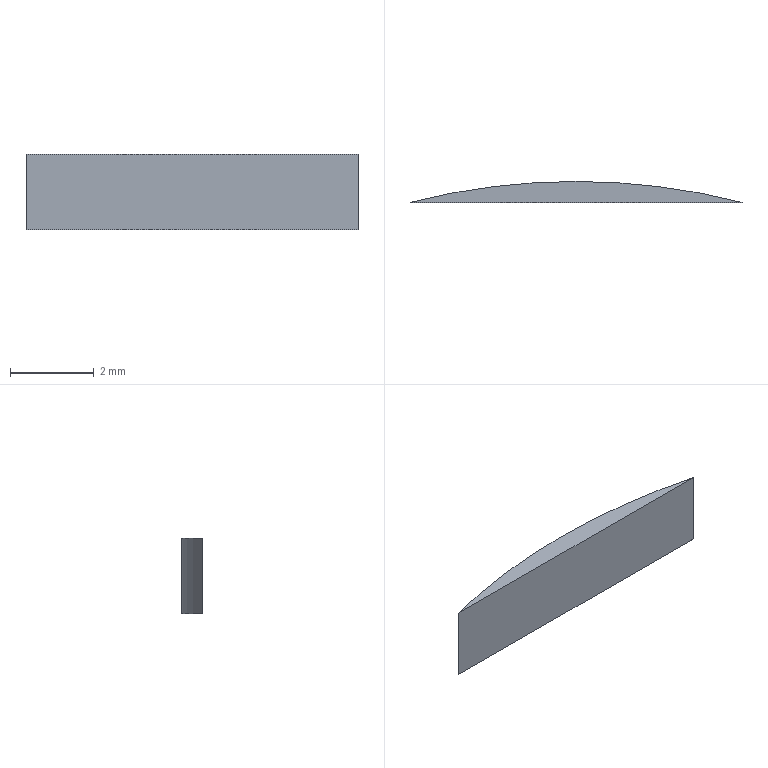Part | STEP file | ASND-0110-Q1-1 | 1 solid | 4 faces | box 7.937 x 0.5 x 1.8 mm | volume 4.777 mm3 | plane 3 | cylinder 1 | commonest cylinder face diameters 32 x1
STEP:
#1=CARTESIAN_POINT('',(0.,0.,0.));
#2=DIRECTION('',(0.,0.,1.));
#3=DIRECTION('',(1.,0.,0.));
#4=AXIS2_PLACEMENT_3D('',#1,#2,#3);
#5=CARTESIAN_POINT('',(2996.031,15.5,-129.5));
#6=VERTEX_POINT('',#5);
#7=CARTESIAN_POINT('',(2996.031,15.5,-127.7));
#8=VERTEX_POINT('',#7);
#9=CARTESIAN_POINT('',(2996.031,15.5,-128.6));
#10=DIRECTION('',(0.,0.,1.));
#11=VECTOR('',#10,1.);
#12=LINE('',#9,#11);
#13=CARTESIAN_POINT('',(3000.,0.,-128.6));
#14=DIRECTION('',(0.,0.,-1.));
#15=DIRECTION('',(-1.,0.,0.));
#16=AXIS2_PLACEMENT_3D('',#13,#14,#15);
#17=CYLINDRICAL_SURFACE('',#16,16.);
#18=CARTESIAN_POINT('',(1.32,0.));
#19=DIRECTION('',(0.,-1.));
#20=VECTOR('',#19,1.);
#21=LINE('',#18,#20);
#22=(GEOMETRIC_REPRESENTATION_CONTEXT(2)PARAMETRIC_REPRESENTATION_CONTEXT()REPRESENTATION_CONTEXT('',''));
#23=DEFINITIONAL_REPRESENTATION('',(#21),#22);
#24=PCURVE('',#17,#23);
#25=CARTESIAN_POINT('',(1241.605,15.5,-583.518));
#26=DIRECTION('',(0.,1.,0.));
#27=DIRECTION('',(0.7071,0.,0.7071));
#28=AXIS2_PLACEMENT_3D('',#25,#26,#27);
#29=PLANE('',#28);
#30=CARTESIAN_POINT('',(1562.242,918.891));
#31=DIRECTION('',(0.7071,-0.7071));
#32=VECTOR('',#31,1.);
#33=LINE('',#30,#32);
#34=(GEOMETRIC_REPRESENTATION_CONTEXT(2)PARAMETRIC_REPRESENTATION_CONTEXT()REPRESENTATION_CONTEXT('',''));
#35=DEFINITIONAL_REPRESENTATION('',(#33),#34);
#36=PCURVE('',#29,#35);
#37=SURFACE_CURVE('',#12,(#24,#36),.PCURVE_S1.);
#38=EDGE_CURVE('',#6,#8,#37,.T.);
#39=ORIENTED_EDGE('',*,*,#38,.T.);
#40=CARTESIAN_POINT('',(3003.969,15.5,-127.7));
#41=VERTEX_POINT('',#40);
#42=CARTESIAN_POINT('',(3000.,0.,-127.7));
#43=DIRECTION('',(0.,0.,-1.));
#44=DIRECTION('',(-1.,0.,0.));
#45=AXIS2_PLACEMENT_3D('',#42,#43,#44);
#46=CIRCLE('',#45,16.);
#47=CARTESIAN_POINT('',(0.,-0.9));
#48=DIRECTION('',(1.,0.));
#49=VECTOR('',#48,1.);
#50=LINE('',#47,#49);
#51=(GEOMETRIC_REPRESENTATION_CONTEXT(2)PARAMETRIC_REPRESENTATION_CONTEXT()REPRESENTATION_CONTEXT('',''));
#52=DEFINITIONAL_REPRESENTATION('',(#50),#51);
#53=PCURVE('',#17,#52);
#54=CARTESIAN_POINT('',(3000.,14.,-127.7));
#55=DIRECTION('',(0.,0.,1.));
#56=DIRECTION('',(0.7071,0.7071,0.));
#57=AXIS2_PLACEMENT_3D('',#54,#55,#56);
#58=PLANE('',#57);
#59=CARTESIAN_POINT('',(-21.213,1.414));
#60=CARTESIAN_POINT('',(-1.617,21.01));
#61=CARTESIAN_POINT('',(5.555,-5.758));
#62=CARTESIAN_POINT('',(12.728,-32.527));
#63=CARTESIAN_POINT('',(-14.041,-25.354));
#64=CARTESIAN_POINT('',(-40.809,-18.182));
#65=CARTESIAN_POINT('',(-21.213,1.414));
#66=(BOUNDED_CURVE()B_SPLINE_CURVE(2,(#59,#60,#61,#62,#63,#64,#65),.UNSPECIFIED.,.T.,.F.)B_SPLINE_CURVE_WITH_KNOTS((1,2,2,2,2,1),(-2.094,0.,2.094,4.189,6.283,8.378),.UNSPECIFIED.)CURVE()GEOMETRIC_REPRESENTATION_ITEM()RATIONAL_B_SPLINE_CURVE((1.,0.5,1.,0.5,1.,0.5,1.))REPRESENTATION_ITEM(''));
#67=(GEOMETRIC_REPRESENTATION_CONTEXT(2)PARAMETRIC_REPRESENTATION_CONTEXT()REPRESENTATION_CONTEXT('',''));
#68=DEFINITIONAL_REPRESENTATION('',(#66),#67);
#69=PCURVE('',#58,#68);
#70=SURFACE_CURVE('',#46,(#53,#69),.PCURVE_S1.);
#71=EDGE_CURVE('',#8,#41,#70,.T.);
#72=ORIENTED_EDGE('',*,*,#71,.T.);
#73=CARTESIAN_POINT('',(3003.969,15.5,-129.5));
#74=VERTEX_POINT('',#73);
#75=CARTESIAN_POINT('',(3003.969,15.5,-128.6));
#76=DIRECTION('',(0.,0.,-1.));
#77=VECTOR('',#76,1.);
#78=LINE('',#75,#77);
#79=CARTESIAN_POINT('',(1.821,0.));
#80=DIRECTION('',(0.,1.));
#81=VECTOR('',#80,1.);
#82=LINE('',#79,#81);
#83=(GEOMETRIC_REPRESENTATION_CONTEXT(2)PARAMETRIC_REPRESENTATION_CONTEXT()REPRESENTATION_CONTEXT('',''));
#84=DEFINITIONAL_REPRESENTATION('',(#82),#83);
#85=PCURVE('',#17,#84);
#86=CARTESIAN_POINT('',(1567.854,924.504));
#87=DIRECTION('',(-0.7071,0.7071));
#88=VECTOR('',#87,1.);
#89=LINE('',#86,#88);
#90=(GEOMETRIC_REPRESENTATION_CONTEXT(2)PARAMETRIC_REPRESENTATION_CONTEXT()REPRESENTATION_CONTEXT('',''));
#91=DEFINITIONAL_REPRESENTATION('',(#89),#90);
#92=PCURVE('',#29,#91);
#93=SURFACE_CURVE('',#78,(#85,#92),.PCURVE_S1.);
#94=EDGE_CURVE('',#41,#74,#93,.T.);
#95=ORIENTED_EDGE('',*,*,#94,.T.);
#96=CARTESIAN_POINT('',(3000.,0.,-129.5));
#97=DIRECTION('',(0.,0.,-1.));
#98=DIRECTION('',(-1.,0.,0.));
#99=AXIS2_PLACEMENT_3D('',#96,#97,#98);
#100=CIRCLE('',#99,16.);
#101=CARTESIAN_POINT('',(0.,0.9));
#102=DIRECTION('',(1.,0.));
#103=VECTOR('',#102,1.);
#104=LINE('',#101,#103);
#105=(GEOMETRIC_REPRESENTATION_CONTEXT(2)PARAMETRIC_REPRESENTATION_CONTEXT()REPRESENTATION_CONTEXT('',''));
#106=DEFINITIONAL_REPRESENTATION('',(#104),#105);
#107=PCURVE('',#17,#106);
#108=CARTESIAN_POINT('',(3000.,15.75,-129.5));
#109=DIRECTION('',(0.,0.,-1.));
#110=DIRECTION('',(0.7071,0.7071,0.));
#111=AXIS2_PLACEMENT_3D('',#108,#109,#110);
#112=PLANE('',#111);
#113=CARTESIAN_POINT('',(-11.137,11.137));
#114=DIRECTION('',(-0.7071,-0.7071));
#115=AXIS2_PLACEMENT_2D('',#113,#114);
#116=CIRCLE('',#115,16.);
#117=(GEOMETRIC_REPRESENTATION_CONTEXT(2)PARAMETRIC_REPRESENTATION_CONTEXT()REPRESENTATION_CONTEXT('',''));
#118=DEFINITIONAL_REPRESENTATION('',(#116),#117);
#119=PCURVE('',#112,#118);
#120=SURFACE_CURVE('',#100,(#107,#119),.PCURVE_S1.);
#121=EDGE_CURVE('',#6,#74,#120,.T.);
#122=ORIENTED_EDGE('',*,*,#121,.F.);
#123=EDGE_LOOP('',(#39,#72,#95,#122));
#124=FACE_BOUND('',#123,.T.);
#125=ADVANCED_FACE('',(#124),#17,.T.);
#126=CARTESIAN_POINT('',(2120.803,15.5,-129.5));
#127=DIRECTION('',(-1.,0.,0.));
#128=VECTOR('',#127,1.);
#129=LINE('',#126,#128);
#130=CARTESIAN_POINT('',(-621.863,-621.51));
#131=DIRECTION('',(-0.7071,-0.7071));
#132=VECTOR('',#131,1.);
#133=LINE('',#130,#132);
#134=(GEOMETRIC_REPRESENTATION_CONTEXT(2)PARAMETRIC_REPRESENTATION_CONTEXT()REPRESENTATION_CONTEXT('',''));
#135=DEFINITIONAL_REPRESENTATION('',(#133),#134);
#136=PCURVE('',#112,#135);
#137=CARTESIAN_POINT('',(942.725,300.647));
#138=DIRECTION('',(-0.7071,-0.7071));
#139=VECTOR('',#138,1.);
#140=LINE('',#137,#139);
#141=(GEOMETRIC_REPRESENTATION_CONTEXT(2)PARAMETRIC_REPRESENTATION_CONTEXT()REPRESENTATION_CONTEXT('',''));
#142=DEFINITIONAL_REPRESENTATION('',(#140),#141);
#143=PCURVE('',#29,#142);
#144=SURFACE_CURVE('',#129,(#136,#143),.PCURVE_S1.);
#145=EDGE_CURVE('',#74,#6,#144,.T.);
#146=ORIENTED_EDGE('',*,*,#145,.T.);
#147=ORIENTED_EDGE('',*,*,#121,.T.);
#148=EDGE_LOOP('',(#146,#147));
#149=FACE_BOUND('',#148,.T.);
#150=ADVANCED_FACE('',(#149),#112,.T.);
#151=CARTESIAN_POINT('',(2120.803,15.5,-127.7));
#152=DIRECTION('',(1.,0.,0.));
#153=VECTOR('',#152,1.);
#154=LINE('',#151,#153);
#155=CARTESIAN_POINT('',(-620.626,622.747));
#156=DIRECTION('',(0.7071,-0.7071));
#157=VECTOR('',#156,1.);
#158=LINE('',#155,#157);
#159=(GEOMETRIC_REPRESENTATION_CONTEXT(2)PARAMETRIC_REPRESENTATION_CONTEXT()REPRESENTATION_CONTEXT('',''));
#160=DEFINITIONAL_REPRESENTATION('',(#158),#159);
#161=PCURVE('',#58,#160);
#162=CARTESIAN_POINT('',(943.998,299.375));
#163=DIRECTION('',(0.7071,0.7071));
#164=VECTOR('',#163,1.);
#165=LINE('',#162,#164);
#166=(GEOMETRIC_REPRESENTATION_CONTEXT(2)PARAMETRIC_REPRESENTATION_CONTEXT()REPRESENTATION_CONTEXT('',''));
#167=DEFINITIONAL_REPRESENTATION('',(#165),#166);
#168=PCURVE('',#29,#167);
#169=SURFACE_CURVE('',#154,(#161,#168),.PCURVE_S1.);
#170=EDGE_CURVE('',#8,#41,#169,.T.);
#171=ORIENTED_EDGE('',*,*,#170,.T.);
#172=ORIENTED_EDGE('',*,*,#71,.F.);
#173=EDGE_LOOP('',(#171,#172));
#174=FACE_BOUND('',#173,.T.);
#175=ADVANCED_FACE('',(#174),#58,.T.);
#176=ORIENTED_EDGE('',*,*,#145,.F.);
#177=ORIENTED_EDGE('',*,*,#94,.F.);
#178=ORIENTED_EDGE('',*,*,#170,.F.);
#179=ORIENTED_EDGE('',*,*,#38,.F.);
#180=EDGE_LOOP('',(#176,#177,#178,#179));
#181=FACE_BOUND('',#180,.T.);
#182=ADVANCED_FACE('',(#181),#29,.F.);
#183=CLOSED_SHELL('',(#125,#150,#175,#182));
#184=MANIFOLD_SOLID_BREP('',#183);
#185=(LENGTH_UNIT()NAMED_UNIT(*)SI_UNIT(.MILLI.,.METRE.));
#186=UNCERTAINTY_MEASURE_WITH_UNIT(LENGTH_MEASURE(0.0000001),#185,'','');
#187=(NAMED_UNIT(*)PLANE_ANGLE_UNIT()SI_UNIT($,.RADIAN.));
#188=(NAMED_UNIT(*)SI_UNIT($,.STERADIAN.)SOLID_ANGLE_UNIT());
#189=(GEOMETRIC_REPRESENTATION_CONTEXT(3)GLOBAL_UNCERTAINTY_ASSIGNED_CONTEXT((#186))GLOBAL_UNIT_ASSIGNED_CONTEXT((#185,#187,#188))REPRESENTATION_CONTEXT('',''));
#190=ADVANCED_BREP_SHAPE_REPRESENTATION('',(#4,#184),#189);